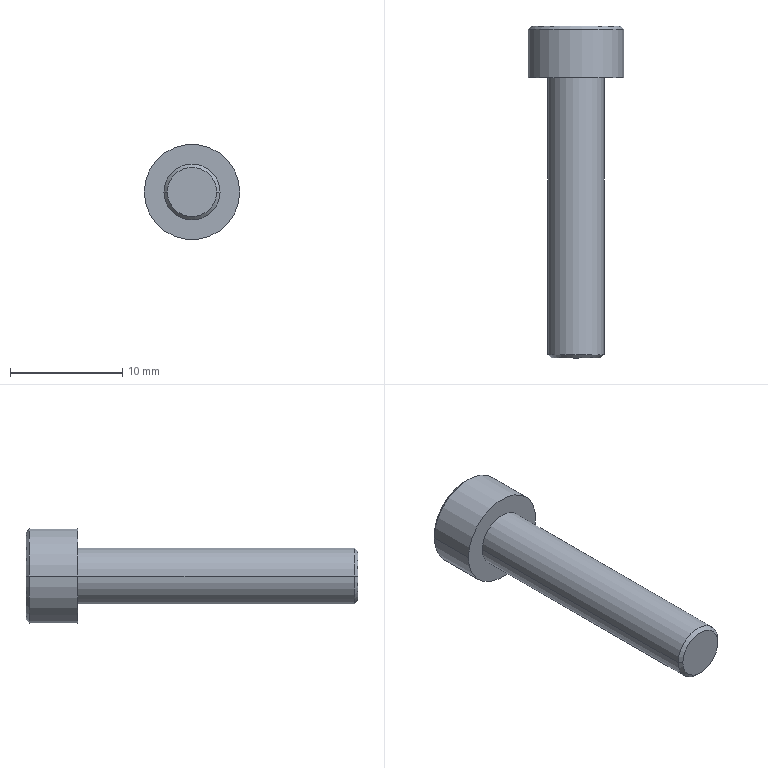Part | NX | 1 solid | 80 faces | box 8.5 x 29.6 x 8.5 mm | volume 703.389 mm3 | plane 70 | cone 6 | cylinder 4 | commonest cylinder face diameters 5 x2 8.5 x2